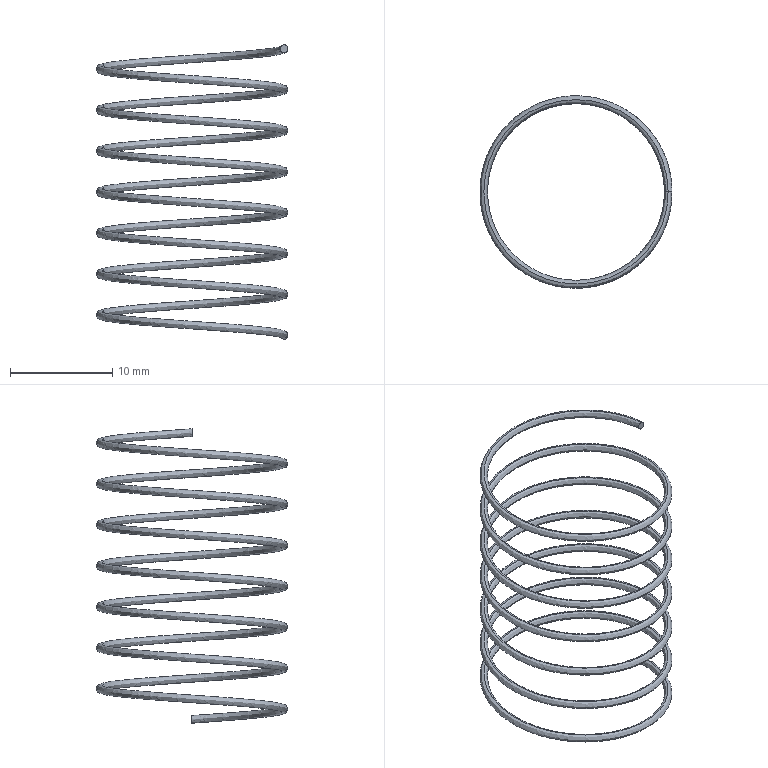Part | STEP file | Spring-rotor test | 1 solid | 4 faces | box 18.75 x 18.75 x 28.75 mm | volume 175.083 mm3 | spline 2 | plane 2